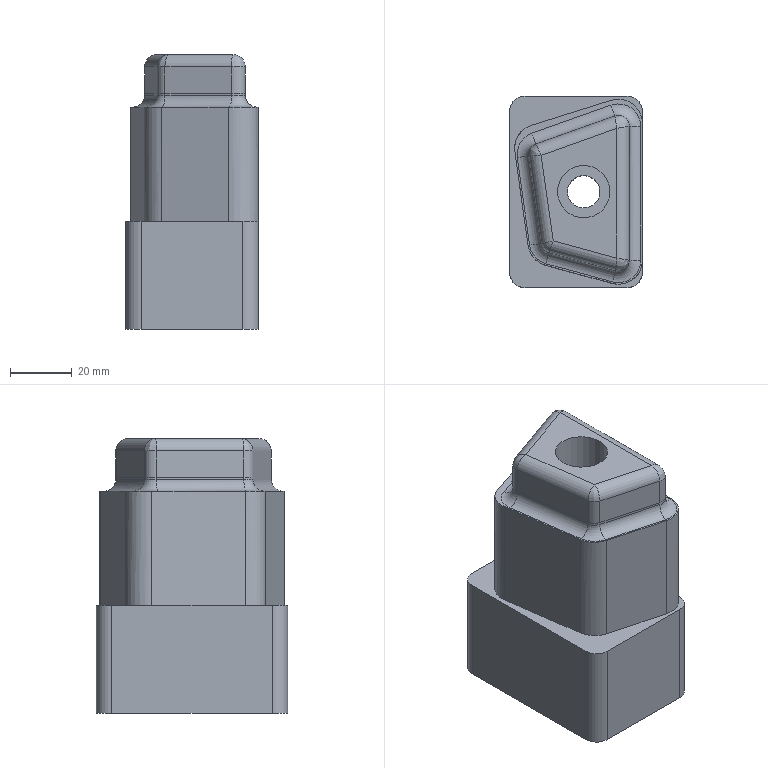Part | STEP file | gslz 2016.10.28-6_id26_x_t | 1 solid | 54 faces | box 43 x 62 x 89 mm | volume 180403 mm3 | cylinder 22 | plane 20 | spline 8 | torus 4 | commonest cylinder face diameters 7 x8 7.5 x4 8 x4 10 x4 10.5 x1 17 x1